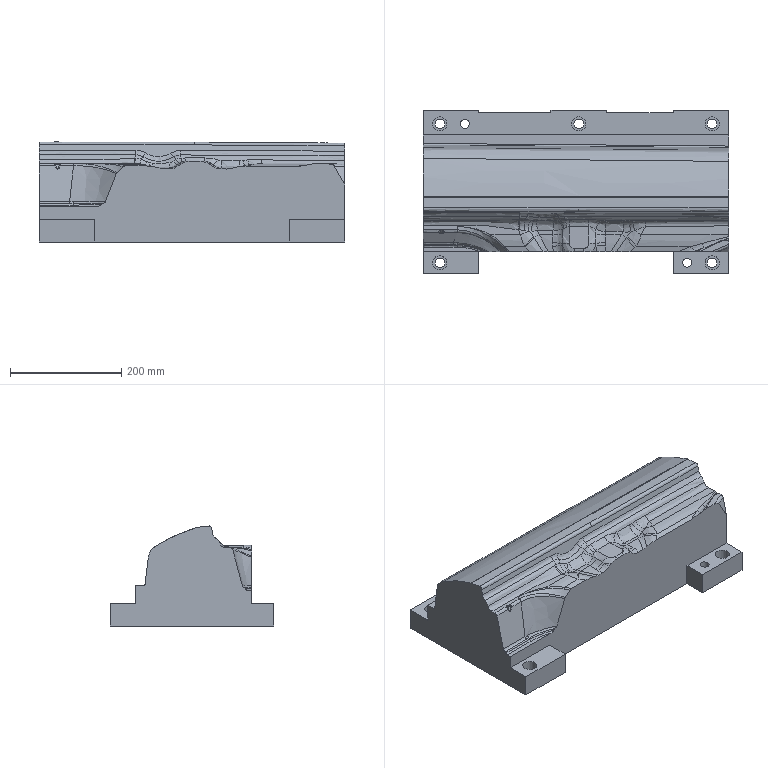Part | NX | features solid 2 | 1 solid | 170 faces | box 550.001 x 295 x 179.996 mm | volume 13679023 mm3 | spline 124 | plane 34 | cylinder 12 | commonest cylinder face diameters 17.5 x5 25.5 x5 16 x2